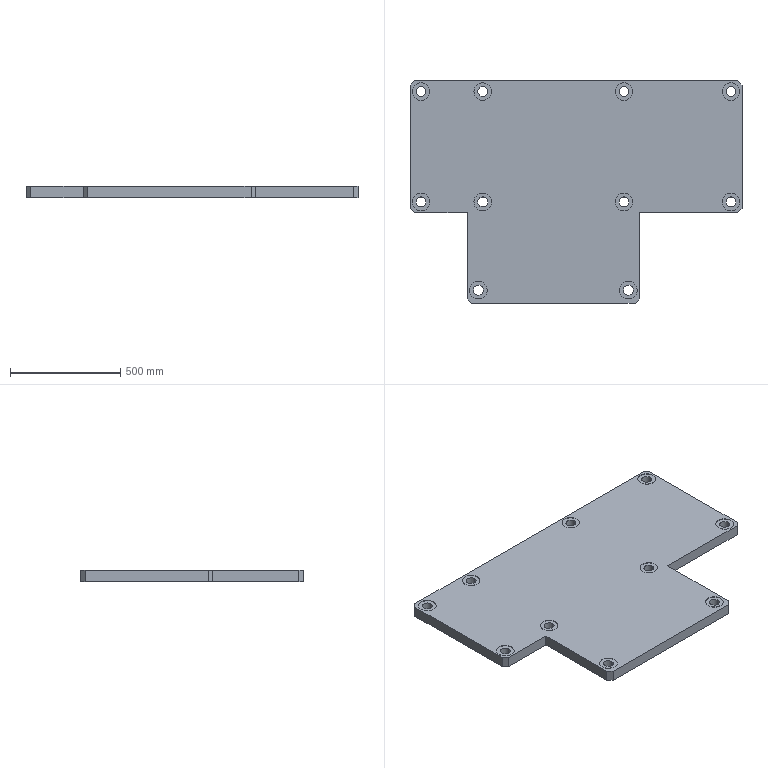Part | SolidWorks | features Chamfer 1, Extrusion 1, HoleWzd 1 | 1 solid | 66 faces | box 1505 x 1010 x 50 mm | volume 60216062 mm3 | cylinder 40 | plane 26 | commonest cylinder face diameters 45 x20 80 x20